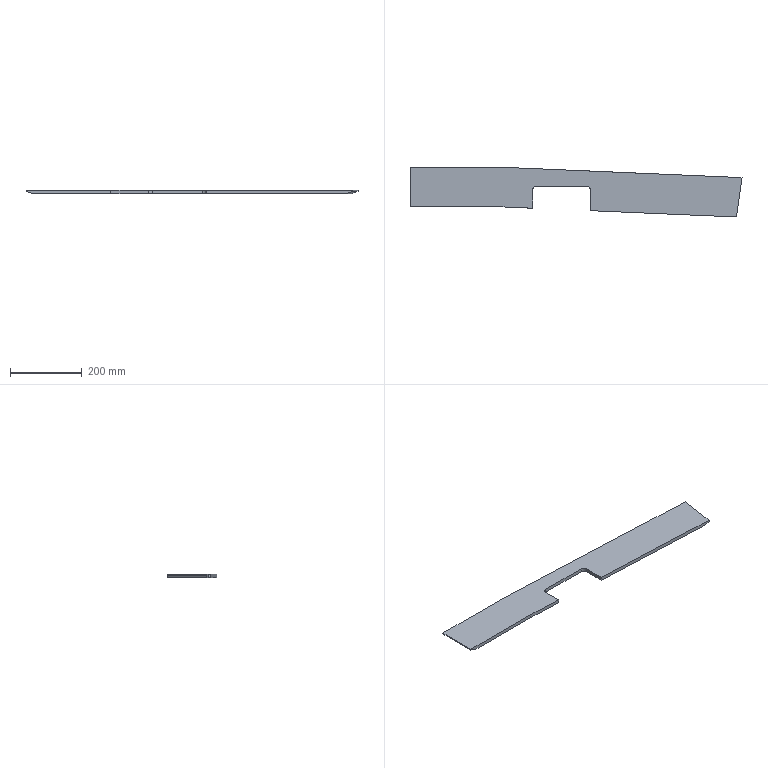Part | SolidWorks | features Chamfer 1, FlatPattern 1, SMBaseFlange 1, SheetMetal 1 | 1 solid | 16 faces | box 922.9 x 138.9 x 10 mm | volume 889368 mm3 | plane 14 | cylinder 2 | commonest cylinder face diameters 20 x2
STEP:
#1=CARTESIAN_POINT('',(0.,110.,-3.));
#2=VERTEX_POINT('',#1);
#3=CARTESIAN_POINT('',(0.,110.,0.));
#4=VERTEX_POINT('',#3);
#5=CARTESIAN_POINT('',(0.,110.,-10.));
#6=DIRECTION('',(0.,0.,1.));
#7=VECTOR('',#6,1000.);
#8=LINE('',#5,#7);
#9=EDGE_CURVE('',#2,#4,#8,.T.);
#10=ORIENTED_EDGE('',*,*,#9,.F.);
#11=CARTESIAN_POINT('',(0.,0.,-3.));
#12=VERTEX_POINT('',#11);
#13=CARTESIAN_POINT('',(0.,0.,-3.));
#14=DIRECTION('',(0.,-1.,0.));
#15=VECTOR('',#14,1000.);
#16=LINE('',#13,#15);
#17=EDGE_CURVE('',#2,#12,#16,.T.);
#18=ORIENTED_EDGE('',*,*,#17,.T.);
#19=CARTESIAN_POINT('',(0.,0.,0.));
#20=VERTEX_POINT('',#19);
#21=CARTESIAN_POINT('',(0.,0.,-10.));
#22=DIRECTION('',(0.,0.,1.));
#23=VECTOR('',#22,1000.);
#24=LINE('',#21,#23);
#25=EDGE_CURVE('',#12,#20,#24,.T.);
#26=ORIENTED_EDGE('',*,*,#25,.T.);
#27=CARTESIAN_POINT('',(0.,0.,0.));
#28=DIRECTION('',(0.,-1.,0.));
#29=VECTOR('',#28,1000.);
#30=LINE('',#27,#29);
#31=EDGE_CURVE('',#4,#20,#30,.T.);
#32=ORIENTED_EDGE('',*,*,#31,.F.);
#33=EDGE_LOOP('',(#10,#18,#26,#32));
#34=FACE_OUTER_BOUND('',#33,.T.);
#35=CARTESIAN_POINT('',(0.,0.,-10.));
#36=DIRECTION('',(-1.,0.,0.));
#37=DIRECTION('',(0.,0.,1.));
#38=AXIS2_PLACEMENT_3D('',#35,#36,#37);
#39=PLANE('',#38);
#40=ADVANCED_FACE('',(#34),#39,.T.);
#41=CARTESIAN_POINT('',(241.26,110.,-10.));
#42=VERTEX_POINT('',#41);
#43=CARTESIAN_POINT('',(20.,110.,-10.));
#44=VERTEX_POINT('',#43);
#45=CARTESIAN_POINT('',(0.,110.,-10.));
#46=DIRECTION('',(-1.,0.,0.));
#47=VECTOR('',#46,1000.);
#48=LINE('',#45,#47);
#49=EDGE_CURVE('',#42,#44,#48,.T.);
#50=ORIENTED_EDGE('',*,*,#49,.T.);
#51=CARTESIAN_POINT('',(2.183,110.,-3.764));
#52=DIRECTION('',(-0.9439,0.,0.3304));
#53=VECTOR('',#52,1000.);
#54=LINE('',#51,#53);
#55=EDGE_CURVE('',#44,#2,#54,.T.);
#56=ORIENTED_EDGE('',*,*,#55,.T.);
#57=ORIENTED_EDGE('',*,*,#9,.T.);
#58=CARTESIAN_POINT('',(241.26,110.,0.));
#59=VERTEX_POINT('',#58);
#60=CARTESIAN_POINT('',(0.,110.,0.));
#61=DIRECTION('',(-1.,0.,0.));
#62=VECTOR('',#61,1000.);
#63=LINE('',#60,#62);
#64=EDGE_CURVE('',#59,#4,#63,.T.);
#65=ORIENTED_EDGE('',*,*,#64,.F.);
#66=CARTESIAN_POINT('',(241.26,110.,-10.));
#67=DIRECTION('',(0.,0.,1.));
#68=VECTOR('',#67,1000.);
#69=LINE('',#66,#68);
#70=EDGE_CURVE('',#42,#59,#69,.T.);
#71=ORIENTED_EDGE('',*,*,#70,.F.);
#72=EDGE_LOOP('',(#50,#56,#57,#65,#71));
#73=FACE_OUTER_BOUND('',#72,.T.);
#74=CARTESIAN_POINT('',(0.,110.,-10.));
#75=DIRECTION('',(0.,1.,0.));
#76=DIRECTION('',(0.,0.,1.));
#77=AXIS2_PLACEMENT_3D('',#74,#75,#76);
#78=PLANE('',#77);
#79=ADVANCED_FACE('',(#73),#78,.T.);
#80=CARTESIAN_POINT('',(922.9,80.677,-3.));
#81=VERTEX_POINT('',#80);
#82=CARTESIAN_POINT('',(922.9,80.677,0.));
#83=VERTEX_POINT('',#82);
#84=CARTESIAN_POINT('',(922.9,80.677,-10.));
#85=DIRECTION('',(0.,0.,1.));
#86=VECTOR('',#85,1000.);
#87=LINE('',#84,#86);
#88=EDGE_CURVE('',#81,#83,#87,.T.);
#89=ORIENTED_EDGE('',*,*,#88,.F.);
#90=CARTESIAN_POINT('',(902.825,81.54,-10.));
#91=VERTEX_POINT('',#90);
#92=CARTESIAN_POINT('',(312.858,106.92,-215.715));
#93=DIRECTION('',(-0.9435,0.04059,-0.329));
#94=VECTOR('',#93,1000.);
#95=LINE('',#92,#94);
#96=EDGE_CURVE('',#81,#91,#95,.T.);
#97=ORIENTED_EDGE('',*,*,#96,.T.);
#98=CARTESIAN_POINT('',(241.26,110.,-10.));
#99=DIRECTION('',(-0.9991,0.04298,0.));
#100=VECTOR('',#99,1000.);
#101=LINE('',#98,#100);
#102=EDGE_CURVE('',#91,#42,#101,.T.);
#103=ORIENTED_EDGE('',*,*,#102,.T.);
#104=ORIENTED_EDGE('',*,*,#70,.T.);
#105=CARTESIAN_POINT('',(241.26,110.,0.));
#106=DIRECTION('',(-0.9991,0.04298,0.));
#107=VECTOR('',#106,1000.);
#108=LINE('',#105,#107);
#109=EDGE_CURVE('',#83,#59,#108,.T.);
#110=ORIENTED_EDGE('',*,*,#109,.F.);
#111=EDGE_LOOP('',(#89,#97,#103,#104,#110));
#112=FACE_OUTER_BOUND('',#111,.T.);
#113=CARTESIAN_POINT('',(241.26,110.,-10.));
#114=DIRECTION('',(0.04298,0.9991,0.));
#115=DIRECTION('',(-0.9991,0.04298,0.));
#116=AXIS2_PLACEMENT_3D('',#113,#114,#115);
#117=PLANE('',#116);
#118=ADVANCED_FACE('',(#112),#117,.T.);
#119=CARTESIAN_POINT('',(907.5,-28.9,-3.));
#120=VERTEX_POINT('',#119);
#121=CARTESIAN_POINT('',(907.5,-28.9,0.));
#122=VERTEX_POINT('',#121);
#123=CARTESIAN_POINT('',(907.5,-28.9,-10.));
#124=DIRECTION('',(0.,0.,1.));
#125=VECTOR('',#124,1000.);
#126=LINE('',#123,#125);
#127=EDGE_CURVE('',#120,#122,#126,.T.);
#128=ORIENTED_EDGE('',*,*,#127,.F.);
#129=CARTESIAN_POINT('',(922.9,80.677,-3.));
#130=DIRECTION('',(0.1392,0.9903,0.));
#131=VECTOR('',#130,1000.);
#132=LINE('',#129,#131);
#133=EDGE_CURVE('',#120,#81,#132,.T.);
#134=ORIENTED_EDGE('',*,*,#133,.T.);
#135=ORIENTED_EDGE('',*,*,#88,.T.);
#136=CARTESIAN_POINT('',(907.5,-28.9,0.));
#137=DIRECTION('',(0.1392,0.9903,0.));
#138=VECTOR('',#137,1000.);
#139=LINE('',#136,#138);
#140=EDGE_CURVE('',#122,#83,#139,.T.);
#141=ORIENTED_EDGE('',*,*,#140,.F.);
#142=EDGE_LOOP('',(#128,#134,#135,#141));
#143=FACE_OUTER_BOUND('',#142,.T.);
#144=CARTESIAN_POINT('',(907.5,-28.9,-10.));
#145=DIRECTION('',(0.9903,-0.1392,0.));
#146=DIRECTION('',(0.1392,0.9903,0.));
#147=AXIS2_PLACEMENT_3D('',#144,#145,#146);
#148=PLANE('',#147);
#149=ADVANCED_FACE('',(#143),#148,.T.);
#150=CARTESIAN_POINT('',(501.,-11.413,-10.));
#151=VERTEX_POINT('',#150);
#152=CARTESIAN_POINT('',(887.425,-28.036,-10.));
#153=VERTEX_POINT('',#152);
#154=CARTESIAN_POINT('',(501.,-11.413,-10.));
#155=DIRECTION('',(0.9991,-0.04298,0.));
#156=VECTOR('',#155,1000.);
#157=LINE('',#154,#156);
#158=EDGE_CURVE('',#151,#153,#157,.T.);
#159=ORIENTED_EDGE('',*,*,#158,.T.);
#160=CARTESIAN_POINT('',(542.821,-13.212,-130.16));
#161=DIRECTION('',(0.9435,-0.04059,0.329));
#162=VECTOR('',#161,1000.);
#163=LINE('',#160,#162);
#164=EDGE_CURVE('',#153,#120,#163,.T.);
#165=ORIENTED_EDGE('',*,*,#164,.T.);
#166=ORIENTED_EDGE('',*,*,#127,.T.);
#167=CARTESIAN_POINT('',(501.,-11.413,0.));
#168=VERTEX_POINT('',#167);
#169=CARTESIAN_POINT('',(501.,-11.413,0.));
#170=DIRECTION('',(0.9991,-0.04298,0.));
#171=VECTOR('',#170,1000.);
#172=LINE('',#169,#171);
#173=EDGE_CURVE('',#168,#122,#172,.T.);
#174=ORIENTED_EDGE('',*,*,#173,.F.);
#175=CARTESIAN_POINT('',(501.,-11.413,-10.));
#176=DIRECTION('',(0.,0.,1.));
#177=VECTOR('',#176,1000.);
#178=LINE('',#175,#177);
#179=EDGE_CURVE('',#151,#168,#178,.T.);
#180=ORIENTED_EDGE('',*,*,#179,.F.);
#181=EDGE_LOOP('',(#159,#165,#166,#174,#180));
#182=FACE_OUTER_BOUND('',#181,.T.);
#183=CARTESIAN_POINT('',(501.,-11.413,-10.));
#184=DIRECTION('',(-0.04298,-0.9991,0.));
#185=DIRECTION('',(0.9991,-0.04298,0.));
#186=AXIS2_PLACEMENT_3D('',#183,#184,#185);
#187=PLANE('',#186);
#188=ADVANCED_FACE('',(#182),#187,.T.);
#189=CARTESIAN_POINT('',(501.,47.,0.));
#190=VERTEX_POINT('',#189);
#191=CARTESIAN_POINT('',(501.,47.,0.));
#192=DIRECTION('',(0.,-1.,0.));
#193=VECTOR('',#192,1000.);
#194=LINE('',#191,#193);
#195=EDGE_CURVE('',#190,#168,#194,.T.);
#196=ORIENTED_EDGE('',*,*,#195,.F.);
#197=CARTESIAN_POINT('',(501.,47.,-10.));
#198=VERTEX_POINT('',#197);
#199=CARTESIAN_POINT('',(501.,47.,-10.));
#200=DIRECTION('',(0.,0.,1.));
#201=VECTOR('',#200,1000.);
#202=LINE('',#199,#201);
#203=EDGE_CURVE('',#198,#190,#202,.T.);
#204=ORIENTED_EDGE('',*,*,#203,.F.);
#205=CARTESIAN_POINT('',(501.,47.,-10.));
#206=DIRECTION('',(0.,-1.,0.));
#207=VECTOR('',#206,1000.);
#208=LINE('',#205,#207);
#209=EDGE_CURVE('',#198,#151,#208,.T.);
#210=ORIENTED_EDGE('',*,*,#209,.T.);
#211=ORIENTED_EDGE('',*,*,#179,.T.);
#212=EDGE_LOOP('',(#196,#204,#210,#211));
#213=FACE_OUTER_BOUND('',#212,.T.);
#214=CARTESIAN_POINT('',(501.,47.,-10.));
#215=DIRECTION('',(-1.,0.,0.));
#216=DIRECTION('',(0.,0.,1.));
#217=AXIS2_PLACEMENT_3D('',#214,#215,#216);
#218=PLANE('',#217);
#219=ADVANCED_FACE('',(#213),#218,.T.);
#220=CARTESIAN_POINT('',(491.,57.,0.));
#221=VERTEX_POINT('',#220);
#222=CARTESIAN_POINT('',(491.,47.,0.));
#223=DIRECTION('',(0.,0.,-1.));
#224=DIRECTION('',(1.,0.,0.));
#225=AXIS2_PLACEMENT_3D('',#222,#223,#224);
#226=CIRCLE('',#225,10.);
#227=EDGE_CURVE('',#221,#190,#226,.T.);
#228=ORIENTED_EDGE('',*,*,#227,.F.);
#229=CARTESIAN_POINT('',(491.,57.,-10.));
#230=VERTEX_POINT('',#229);
#231=CARTESIAN_POINT('',(491.,57.,-10.));
#232=DIRECTION('',(0.,0.,1.));
#233=VECTOR('',#232,1000.);
#234=LINE('',#231,#233);
#235=EDGE_CURVE('',#230,#221,#234,.T.);
#236=ORIENTED_EDGE('',*,*,#235,.F.);
#237=CARTESIAN_POINT('',(491.,47.,-10.));
#238=DIRECTION('',(0.,0.,-1.));
#239=DIRECTION('',(1.,0.,0.));
#240=AXIS2_PLACEMENT_3D('',#237,#238,#239);
#241=CIRCLE('',#240,10.);
#242=EDGE_CURVE('',#230,#198,#241,.T.);
#243=ORIENTED_EDGE('',*,*,#242,.T.);
#244=ORIENTED_EDGE('',*,*,#203,.T.);
#245=EDGE_LOOP('',(#228,#236,#243,#244));
#246=FACE_OUTER_BOUND('',#245,.T.);
#247=CARTESIAN_POINT('',(491.,47.,-10.));
#248=DIRECTION('',(0.,0.,1.));
#249=DIRECTION('',(1.,0.,0.));
#250=AXIS2_PLACEMENT_3D('',#247,#248,#249);
#251=CYLINDRICAL_SURFACE('',#250,10.);
#252=ADVANCED_FACE('',(#246),#251,.F.);
#253=CARTESIAN_POINT('',(351.,57.,0.));
#254=VERTEX_POINT('',#253);
#255=CARTESIAN_POINT('',(351.,57.,0.));
#256=DIRECTION('',(1.,0.,0.));
#257=VECTOR('',#256,1000.);
#258=LINE('',#255,#257);
#259=EDGE_CURVE('',#254,#221,#258,.T.);
#260=ORIENTED_EDGE('',*,*,#259,.F.);
#261=CARTESIAN_POINT('',(351.,57.,-10.));
#262=VERTEX_POINT('',#261);
#263=CARTESIAN_POINT('',(351.,57.,-10.));
#264=DIRECTION('',(0.,0.,1.));
#265=VECTOR('',#264,1000.);
#266=LINE('',#263,#265);
#267=EDGE_CURVE('',#262,#254,#266,.T.);
#268=ORIENTED_EDGE('',*,*,#267,.F.);
#269=CARTESIAN_POINT('',(351.,57.,-10.));
#270=DIRECTION('',(1.,0.,0.));
#271=VECTOR('',#270,1000.);
#272=LINE('',#269,#271);
#273=EDGE_CURVE('',#262,#230,#272,.T.);
#274=ORIENTED_EDGE('',*,*,#273,.T.);
#275=ORIENTED_EDGE('',*,*,#235,.T.);
#276=EDGE_LOOP('',(#260,#268,#274,#275));
#277=FACE_OUTER_BOUND('',#276,.T.);
#278=CARTESIAN_POINT('',(351.,57.,-10.));
#279=DIRECTION('',(0.,-1.,0.));
#280=DIRECTION('',(0.,0.,-1.));
#281=AXIS2_PLACEMENT_3D('',#278,#279,#280);
#282=PLANE('',#281);
#283=ADVANCED_FACE('',(#277),#282,.T.);
#284=CARTESIAN_POINT('',(341.,47.,0.));
#285=VERTEX_POINT('',#284);
#286=CARTESIAN_POINT('',(351.,47.,0.));
#287=DIRECTION('',(0.,0.,-1.));
#288=DIRECTION('',(1.,0.,0.));
#289=AXIS2_PLACEMENT_3D('',#286,#287,#288);
#290=CIRCLE('',#289,10.);
#291=EDGE_CURVE('',#285,#254,#290,.T.);
#292=ORIENTED_EDGE('',*,*,#291,.F.);
#293=CARTESIAN_POINT('',(341.,47.,-10.));
#294=VERTEX_POINT('',#293);
#295=CARTESIAN_POINT('',(341.,47.,-10.));
#296=DIRECTION('',(0.,0.,1.));
#297=VECTOR('',#296,1000.);
#298=LINE('',#295,#297);
#299=EDGE_CURVE('',#294,#285,#298,.T.);
#300=ORIENTED_EDGE('',*,*,#299,.F.);
#301=CARTESIAN_POINT('',(351.,47.,-10.));
#302=DIRECTION('',(0.,0.,-1.));
#303=DIRECTION('',(1.,0.,0.));
#304=AXIS2_PLACEMENT_3D('',#301,#302,#303);
#305=CIRCLE('',#304,10.);
#306=EDGE_CURVE('',#294,#262,#305,.T.);
#307=ORIENTED_EDGE('',*,*,#306,.T.);
#308=ORIENTED_EDGE('',*,*,#267,.T.);
#309=EDGE_LOOP('',(#292,#300,#307,#308));
#310=FACE_OUTER_BOUND('',#309,.T.);
#311=CARTESIAN_POINT('',(351.,47.,-10.));
#312=DIRECTION('',(0.,0.,1.));
#313=DIRECTION('',(1.,0.,0.));
#314=AXIS2_PLACEMENT_3D('',#311,#312,#313);
#315=CYLINDRICAL_SURFACE('',#314,10.);
#316=ADVANCED_FACE('',(#310),#315,.F.);
#317=CARTESIAN_POINT('',(341.,-4.53,0.));
#318=VERTEX_POINT('',#317);
#319=CARTESIAN_POINT('',(341.,-4.53,0.));
#320=DIRECTION('',(0.,1.,0.));
#321=VECTOR('',#320,1000.);
#322=LINE('',#319,#321);
#323=EDGE_CURVE('',#318,#285,#322,.T.);
#324=ORIENTED_EDGE('',*,*,#323,.F.);
#325=CARTESIAN_POINT('',(341.,-4.53,-10.));
#326=VERTEX_POINT('',#325);
#327=CARTESIAN_POINT('',(341.,-4.53,-10.));
#328=DIRECTION('',(0.,0.,1.));
#329=VECTOR('',#328,1000.);
#330=LINE('',#327,#329);
#331=EDGE_CURVE('',#326,#318,#330,.T.);
#332=ORIENTED_EDGE('',*,*,#331,.F.);
#333=CARTESIAN_POINT('',(341.,-4.53,-10.));
#334=DIRECTION('',(0.,1.,0.));
#335=VECTOR('',#334,1000.);
#336=LINE('',#333,#335);
#337=EDGE_CURVE('',#326,#294,#336,.T.);
#338=ORIENTED_EDGE('',*,*,#337,.T.);
#339=ORIENTED_EDGE('',*,*,#299,.T.);
#340=EDGE_LOOP('',(#324,#332,#338,#339));
#341=FACE_OUTER_BOUND('',#340,.T.);
#342=CARTESIAN_POINT('',(341.,-4.53,-10.));
#343=DIRECTION('',(1.,0.,0.));
#344=DIRECTION('',(0.,0.,-1.));
#345=AXIS2_PLACEMENT_3D('',#342,#343,#344);
#346=PLANE('',#345);
#347=ADVANCED_FACE('',(#341),#346,.T.);
#348=CARTESIAN_POINT('',(235.7,0.,0.));
#349=VERTEX_POINT('',#348);
#350=CARTESIAN_POINT('',(235.7,0.,0.));
#351=DIRECTION('',(0.9991,-0.04298,0.));
#352=VECTOR('',#351,1000.);
#353=LINE('',#350,#352);
#354=EDGE_CURVE('',#349,#318,#353,.T.);
#355=ORIENTED_EDGE('',*,*,#354,.F.);
#356=CARTESIAN_POINT('',(235.7,0.,-10.));
#357=VERTEX_POINT('',#356);
#358=CARTESIAN_POINT('',(235.7,0.,-10.));
#359=DIRECTION('',(0.,0.,1.));
#360=VECTOR('',#359,1000.);
#361=LINE('',#358,#360);
#362=EDGE_CURVE('',#357,#349,#361,.T.);
#363=ORIENTED_EDGE('',*,*,#362,.F.);
#364=CARTESIAN_POINT('',(235.7,0.,-10.));
#365=DIRECTION('',(0.9991,-0.04298,0.));
#366=VECTOR('',#365,1000.);
#367=LINE('',#364,#366);
#368=EDGE_CURVE('',#357,#326,#367,.T.);
#369=ORIENTED_EDGE('',*,*,#368,.T.);
#370=ORIENTED_EDGE('',*,*,#331,.T.);
#371=EDGE_LOOP('',(#355,#363,#369,#370));
#372=FACE_OUTER_BOUND('',#371,.T.);
#373=CARTESIAN_POINT('',(235.7,0.,-10.));
#374=DIRECTION('',(-0.04298,-0.9991,0.));
#375=DIRECTION('',(0.9991,-0.04298,0.));
#376=AXIS2_PLACEMENT_3D('',#373,#374,#375);
#377=PLANE('',#376);
#378=ADVANCED_FACE('',(#372),#377,.T.);
#379=ORIENTED_EDGE('',*,*,#25,.F.);
#380=CARTESIAN_POINT('',(20.,0.,-10.));
#381=VERTEX_POINT('',#380);
#382=CARTESIAN_POINT('',(2.183,0.,-3.764));
#383=DIRECTION('',(0.9439,0.,-0.3304));
#384=VECTOR('',#383,1000.);
#385=LINE('',#382,#384);
#386=EDGE_CURVE('',#12,#381,#385,.T.);
#387=ORIENTED_EDGE('',*,*,#386,.T.);
#388=CARTESIAN_POINT('',(0.,0.,-10.));
#389=DIRECTION('',(1.,0.,0.));
#390=VECTOR('',#389,1000.);
#391=LINE('',#388,#390);
#392=EDGE_CURVE('',#381,#357,#391,.T.);
#393=ORIENTED_EDGE('',*,*,#392,.T.);
#394=ORIENTED_EDGE('',*,*,#362,.T.);
#395=CARTESIAN_POINT('',(0.,0.,0.));
#396=DIRECTION('',(1.,0.,0.));
#397=VECTOR('',#396,1000.);
#398=LINE('',#395,#397);
#399=EDGE_CURVE('',#20,#349,#398,.T.);
#400=ORIENTED_EDGE('',*,*,#399,.F.);
#401=EDGE_LOOP('',(#379,#387,#393,#394,#400));
#402=FACE_OUTER_BOUND('',#401,.T.);
#403=CARTESIAN_POINT('',(0.,0.,-10.));
#404=DIRECTION('',(0.,-1.,0.));
#405=DIRECTION('',(0.,0.,-1.));
#406=AXIS2_PLACEMENT_3D('',#403,#404,#405);
#407=PLANE('',#406);
#408=ADVANCED_FACE('',(#402),#407,.T.);
#409=ORIENTED_EDGE('',*,*,#392,.F.);
#410=CARTESIAN_POINT('',(20.,110.,-10.));
#411=DIRECTION('',(0.,1.,0.));
#412=VECTOR('',#411,1000.);
#413=LINE('',#410,#412);
#414=EDGE_CURVE('',#381,#44,#413,.T.);
#415=ORIENTED_EDGE('',*,*,#414,.T.);
#416=ORIENTED_EDGE('',*,*,#49,.F.);
#417=ORIENTED_EDGE('',*,*,#102,.F.);
#418=CARTESIAN_POINT('',(887.695,-26.117,-10.));
#419=DIRECTION('',(-0.1392,-0.9903,0.));
#420=VECTOR('',#419,1000.);
#421=LINE('',#418,#420);
#422=EDGE_CURVE('',#91,#153,#421,.T.);
#423=ORIENTED_EDGE('',*,*,#422,.T.);
#424=ORIENTED_EDGE('',*,*,#158,.F.);
#425=ORIENTED_EDGE('',*,*,#209,.F.);
#426=ORIENTED_EDGE('',*,*,#242,.F.);
#427=ORIENTED_EDGE('',*,*,#273,.F.);
#428=ORIENTED_EDGE('',*,*,#306,.F.);
#429=ORIENTED_EDGE('',*,*,#337,.F.);
#430=ORIENTED_EDGE('',*,*,#368,.F.);
#431=EDGE_LOOP('',(#409,#415,#416,#417,#423,#424,#425,#426,#427,#428,#429,#430));
#432=FACE_OUTER_BOUND('',#431,.T.);
#433=CARTESIAN_POINT('',(491.,47.,-10.));
#434=DIRECTION('',(0.,0.,1.));
#435=DIRECTION('',(1.,0.,0.));
#436=AXIS2_PLACEMENT_3D('',#433,#434,#435);
#437=PLANE('',#436);
#438=ADVANCED_FACE('',(#432),#437,.F.);
#439=ORIENTED_EDGE('',*,*,#31,.T.);
#440=ORIENTED_EDGE('',*,*,#399,.T.);
#441=ORIENTED_EDGE('',*,*,#354,.T.);
#442=ORIENTED_EDGE('',*,*,#323,.T.);
#443=ORIENTED_EDGE('',*,*,#291,.T.);
#444=ORIENTED_EDGE('',*,*,#259,.T.);
#445=ORIENTED_EDGE('',*,*,#227,.T.);
#446=ORIENTED_EDGE('',*,*,#195,.T.);
#447=ORIENTED_EDGE('',*,*,#173,.T.);
#448=ORIENTED_EDGE('',*,*,#140,.T.);
#449=ORIENTED_EDGE('',*,*,#109,.T.);
#450=ORIENTED_EDGE('',*,*,#64,.T.);
#451=EDGE_LOOP('',(#439,#440,#441,#442,#443,#444,#445,#446,#447,#448,#449,#450));
#452=FACE_OUTER_BOUND('',#451,.T.);
#453=CARTESIAN_POINT('',(491.,47.,0.));
#454=DIRECTION('',(0.,0.,1.));
#455=DIRECTION('',(1.,0.,0.));
#456=AXIS2_PLACEMENT_3D('',#453,#454,#455);
#457=PLANE('',#456);
#458=ADVANCED_FACE('',(#452),#457,.T.);
#459=ORIENTED_EDGE('',*,*,#55,.F.);
#460=ORIENTED_EDGE('',*,*,#414,.F.);
#461=ORIENTED_EDGE('',*,*,#386,.F.);
#462=ORIENTED_EDGE('',*,*,#17,.F.);
#463=EDGE_LOOP('',(#459,#460,#461,#462));
#464=FACE_OUTER_BOUND('',#463,.T.);
#465=CARTESIAN_POINT('',(0.,0.,-3.));
#466=DIRECTION('',(-0.3304,0.,-0.9439));
#467=DIRECTION('',(-0.9439,0.,0.3304));
#468=AXIS2_PLACEMENT_3D('',#465,#466,#467);
#469=PLANE('',#468);
#470=ADVANCED_FACE('',(#464),#469,.T.);
#471=ORIENTED_EDGE('',*,*,#164,.F.);
#472=ORIENTED_EDGE('',*,*,#422,.F.);
#473=ORIENTED_EDGE('',*,*,#96,.F.);
#474=ORIENTED_EDGE('',*,*,#133,.F.);
#475=EDGE_LOOP('',(#471,#472,#473,#474));
#476=FACE_OUTER_BOUND('',#475,.T.);
#477=CARTESIAN_POINT('',(907.5,-28.9,-3.));
#478=DIRECTION('',(0.3271,-0.04598,-0.9439));
#479=DIRECTION('',(-0.9449,0.,-0.3275));
#480=AXIS2_PLACEMENT_3D('',#477,#478,#479);
#481=PLANE('',#480);
#482=ADVANCED_FACE('',(#476),#481,.T.);
#483=CLOSED_SHELL('',(#40,#79,#118,#149,#188,#219,#252,#283,#316,#347,#378,#408,#438,#458,#470,#482));
#484=MANIFOLD_SOLID_BREP('',#483);
#485=CARTESIAN_POINT('',(0.,0.,0.));
#486=DIRECTION('',(0.,0.,1.));
#487=DIRECTION('',(1.,0.,0.));
#488=AXIS2_PLACEMENT_3D('',#485,#486,#487);
#489=(LENGTH_UNIT()NAMED_UNIT(*)SI_UNIT(.MILLI.,.METRE.));
#490=UNCERTAINTY_MEASURE_WITH_UNIT(LENGTH_MEASURE(0.00001),#489,'','');
#491=(NAMED_UNIT(*)PLANE_ANGLE_UNIT()SI_UNIT($,.RADIAN.));
#492=(NAMED_UNIT(*)SI_UNIT($,.STERADIAN.)SOLID_ANGLE_UNIT());
#493=(GEOMETRIC_REPRESENTATION_CONTEXT(3)GLOBAL_UNCERTAINTY_ASSIGNED_CONTEXT((#490))GLOBAL_UNIT_ASSIGNED_CONTEXT((#489,#491,#492))REPRESENTATION_CONTEXT('',''));
#494=ADVANCED_BREP_SHAPE_REPRESENTATION('',(#484,#488),#493);